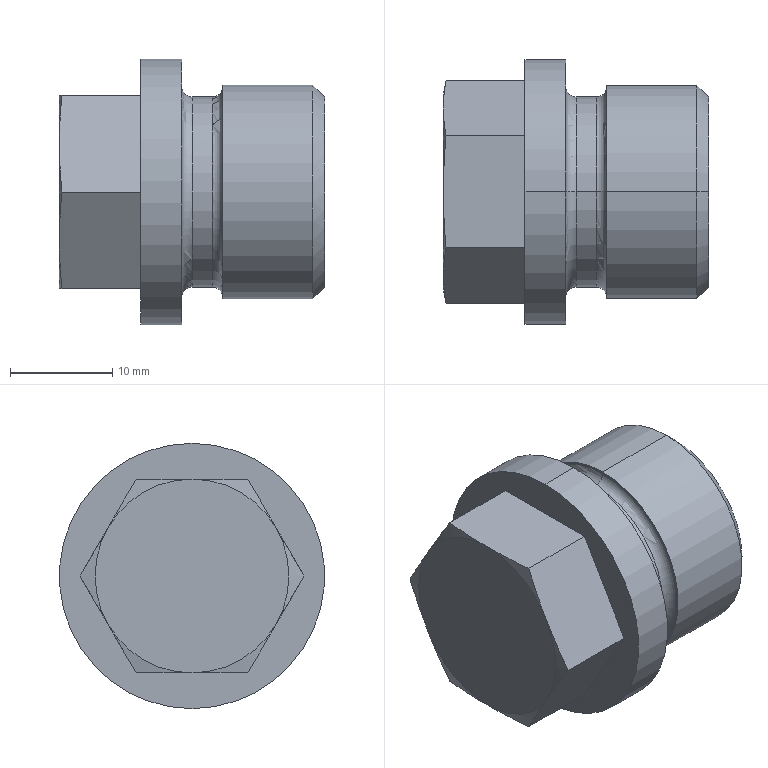Part | SolidWorks | features Boss 1, Cut 1, Fillet 1, Revolution 1 | 1 solid | 29 faces | box 26 x 26 x 26 mm | volume 9145 mm3 | plane 11 | cone 8 | cylinder 6 | torus 4 | commonest cylinder face diameters 18.631 x2 20.955 x2 26 x2
STEP:
#1=CARTESIAN_POINT('',(12.,0.,-10.316));
#2=VERTEX_POINT('',#1);
#3=CARTESIAN_POINT('',(12.,0.,10.316));
#4=VERTEX_POINT('',#3);
#5=CARTESIAN_POINT('',(12.,0.,0.));
#6=DIRECTION('',(-1.,0.,0.));
#7=DIRECTION('',(0.,0.,1.));
#8=AXIS2_PLACEMENT_3D('',#5,#6,#7);
#9=CIRCLE('',#8,10.316);
#10=EDGE_CURVE('',#2,#4,#9,.T.);
#11=ORIENTED_EDGE('',*,*,#10,.F.);
#12=CARTESIAN_POINT('',(13.,0.,-9.316));
#13=VERTEX_POINT('',#12);
#14=CARTESIAN_POINT('',(13.,0.,-10.316));
#15=DIRECTION('',(0.,1.,0.));
#16=DIRECTION('',(0.,0.,1.));
#17=AXIS2_PLACEMENT_3D('',#14,#15,#16);
#18=CIRCLE('',#17,1.);
#19=EDGE_CURVE('',#2,#13,#18,.T.);
#20=ORIENTED_EDGE('',*,*,#19,.T.);
#21=CARTESIAN_POINT('',(13.,0.,9.316));
#22=VERTEX_POINT('',#21);
#23=CARTESIAN_POINT('',(13.,0.,0.));
#24=DIRECTION('',(1.,0.,0.));
#25=DIRECTION('',(0.,0.,1.));
#26=AXIS2_PLACEMENT_3D('',#23,#24,#25);
#27=CIRCLE('',#26,9.316);
#28=EDGE_CURVE('',#22,#13,#27,.T.);
#29=ORIENTED_EDGE('',*,*,#28,.F.);
#30=CARTESIAN_POINT('',(13.,0.,10.316));
#31=DIRECTION('',(0.,-1.,0.));
#32=DIRECTION('',(0.,0.,-1.));
#33=AXIS2_PLACEMENT_3D('',#30,#31,#32);
#34=CIRCLE('',#33,1.);
#35=EDGE_CURVE('',#4,#22,#34,.T.);
#36=ORIENTED_EDGE('',*,*,#35,.F.);
#37=EDGE_LOOP('',(#11,#20,#29,#36));
#38=FACE_OUTER_BOUND('',#37,.T.);
#39=CARTESIAN_POINT('',(13.,0.,0.));
#40=DIRECTION('',(-1.,0.,0.));
#41=DIRECTION('',(0.,0.,1.));
#42=AXIS2_PLACEMENT_3D('',#39,#40,#41);
#43=TOROIDAL_SURFACE('',#42,10.316,1.);
#44=ADVANCED_FACE('',(#38),#43,.F.);
#45=CARTESIAN_POINT('',(16.,0.,10.316));
#46=VERTEX_POINT('',#45);
#47=CARTESIAN_POINT('',(16.,0.,-10.316));
#48=VERTEX_POINT('',#47);
#49=CARTESIAN_POINT('',(16.,0.,0.));
#50=DIRECTION('',(1.,0.,0.));
#51=DIRECTION('',(0.,0.,-1.));
#52=AXIS2_PLACEMENT_3D('',#49,#50,#51);
#53=CIRCLE('',#52,10.316);
#54=EDGE_CURVE('',#46,#48,#53,.T.);
#55=ORIENTED_EDGE('',*,*,#54,.F.);
#56=CARTESIAN_POINT('',(15.,0.,9.316));
#57=VERTEX_POINT('',#56);
#58=CARTESIAN_POINT('',(15.,0.,10.316));
#59=DIRECTION('',(0.,1.,0.));
#60=DIRECTION('',(0.,0.,1.));
#61=AXIS2_PLACEMENT_3D('',#58,#59,#60);
#62=CIRCLE('',#61,1.);
#63=EDGE_CURVE('',#46,#57,#62,.T.);
#64=ORIENTED_EDGE('',*,*,#63,.T.);
#65=CARTESIAN_POINT('',(15.,0.,-9.316));
#66=VERTEX_POINT('',#65);
#67=CARTESIAN_POINT('',(15.,0.,0.));
#68=DIRECTION('',(-1.,0.,0.));
#69=DIRECTION('',(0.,0.,-1.));
#70=AXIS2_PLACEMENT_3D('',#67,#68,#69);
#71=CIRCLE('',#70,9.316);
#72=EDGE_CURVE('',#66,#57,#71,.T.);
#73=ORIENTED_EDGE('',*,*,#72,.F.);
#74=CARTESIAN_POINT('',(15.,0.,-10.316));
#75=DIRECTION('',(0.,-1.,0.));
#76=DIRECTION('',(0.,0.,-1.));
#77=AXIS2_PLACEMENT_3D('',#74,#75,#76);
#78=CIRCLE('',#77,1.);
#79=EDGE_CURVE('',#48,#66,#78,.T.);
#80=ORIENTED_EDGE('',*,*,#79,.F.);
#81=EDGE_LOOP('',(#55,#64,#73,#80));
#82=FACE_OUTER_BOUND('',#81,.T.);
#83=CARTESIAN_POINT('',(15.,0.,0.));
#84=DIRECTION('',(1.,0.,0.));
#85=DIRECTION('',(0.,0.,-1.));
#86=AXIS2_PLACEMENT_3D('',#83,#84,#85);
#87=TOROIDAL_SURFACE('',#86,10.316,1.);
#88=ADVANCED_FACE('',(#82),#87,.F.);
#89=CARTESIAN_POINT('',(26.,0.,9.316));
#90=VERTEX_POINT('',#89);
#91=CARTESIAN_POINT('',(26.,0.,-9.316));
#92=VERTEX_POINT('',#91);
#93=CARTESIAN_POINT('',(26.,0.,0.));
#94=DIRECTION('',(-1.,0.,0.));
#95=DIRECTION('',(0.,0.,1.));
#96=AXIS2_PLACEMENT_3D('',#93,#94,#95);
#97=CIRCLE('',#96,9.316);
#98=EDGE_CURVE('',#90,#92,#97,.T.);
#99=ORIENTED_EDGE('',*,*,#98,.T.);
#100=CARTESIAN_POINT('',(24.838,0.,-10.477));
#101=VERTEX_POINT('',#100);
#102=CARTESIAN_POINT('',(26.,0.,-9.316));
#103=DIRECTION('',(-0.7071,0.,-0.7071));
#104=VECTOR('',#103,1000.);
#105=LINE('',#102,#104);
#106=EDGE_CURVE('',#92,#101,#105,.T.);
#107=ORIENTED_EDGE('',*,*,#106,.T.);
#108=CARTESIAN_POINT('',(24.838,0.,10.477));
#109=VERTEX_POINT('',#108);
#110=CARTESIAN_POINT('',(24.838,0.,0.));
#111=DIRECTION('',(-1.,0.,0.));
#112=DIRECTION('',(0.,0.,1.));
#113=AXIS2_PLACEMENT_3D('',#110,#111,#112);
#114=CIRCLE('',#113,10.477);
#115=EDGE_CURVE('',#109,#101,#114,.T.);
#116=ORIENTED_EDGE('',*,*,#115,.F.);
#117=CARTESIAN_POINT('',(26.,0.,9.316));
#118=DIRECTION('',(-0.7071,0.,0.7071));
#119=VECTOR('',#118,1000.);
#120=LINE('',#117,#119);
#121=EDGE_CURVE('',#90,#109,#120,.T.);
#122=ORIENTED_EDGE('',*,*,#121,.F.);
#123=EDGE_LOOP('',(#99,#107,#116,#122));
#124=FACE_OUTER_BOUND('',#123,.T.);
#125=CARTESIAN_POINT('',(26.,0.,0.));
#126=DIRECTION('',(-1.,0.,0.));
#127=DIRECTION('',(0.,0.,1.));
#128=AXIS2_PLACEMENT_3D('',#125,#126,#127);
#129=CONICAL_SURFACE('',#128,9.316,0.7854);
#130=ADVANCED_FACE('',(#124),#129,.T.);
#131=ORIENTED_EDGE('',*,*,#115,.T.);
#132=CARTESIAN_POINT('',(16.,0.,-10.477));
#133=VERTEX_POINT('',#132);
#134=CARTESIAN_POINT('',(0.,0.,-10.477));
#135=DIRECTION('',(-1.,0.,0.));
#136=VECTOR('',#135,1000.);
#137=LINE('',#134,#136);
#138=EDGE_CURVE('',#101,#133,#137,.T.);
#139=ORIENTED_EDGE('',*,*,#138,.T.);
#140=CARTESIAN_POINT('',(16.,0.,10.477));
#141=VERTEX_POINT('',#140);
#142=CARTESIAN_POINT('',(16.,0.,0.));
#143=DIRECTION('',(-1.,0.,0.));
#144=DIRECTION('',(0.,0.,1.));
#145=AXIS2_PLACEMENT_3D('',#142,#143,#144);
#146=CIRCLE('',#145,10.477);
#147=EDGE_CURVE('',#141,#133,#146,.T.);
#148=ORIENTED_EDGE('',*,*,#147,.F.);
#149=CARTESIAN_POINT('',(0.,0.,10.477));
#150=DIRECTION('',(-1.,0.,0.));
#151=VECTOR('',#150,1000.);
#152=LINE('',#149,#151);
#153=EDGE_CURVE('',#109,#141,#152,.T.);
#154=ORIENTED_EDGE('',*,*,#153,.F.);
#155=EDGE_LOOP('',(#131,#139,#148,#154));
#156=FACE_OUTER_BOUND('',#155,.T.);
#157=CARTESIAN_POINT('',(0.,0.,0.));
#158=DIRECTION('',(-1.,0.,0.));
#159=DIRECTION('',(0.,0.,1.));
#160=AXIS2_PLACEMENT_3D('',#157,#158,#159);
#161=CYLINDRICAL_SURFACE('',#160,10.477);
#162=ADVANCED_FACE('',(#156),#161,.T.);
#163=CARTESIAN_POINT('',(15.,0.,0.));
#164=DIRECTION('',(-1.,0.,0.));
#165=DIRECTION('',(0.,0.,-1.));
#166=AXIS2_PLACEMENT_3D('',#163,#164,#165);
#167=CIRCLE('',#166,9.316);
#168=EDGE_CURVE('',#57,#66,#167,.T.);
#169=ORIENTED_EDGE('',*,*,#168,.T.);
#170=CARTESIAN_POINT('',(0.,0.,-9.316));
#171=DIRECTION('',(-1.,0.,0.));
#172=VECTOR('',#171,1000.);
#173=LINE('',#170,#172);
#174=EDGE_CURVE('',#66,#13,#173,.T.);
#175=ORIENTED_EDGE('',*,*,#174,.T.);
#176=CARTESIAN_POINT('',(13.,0.,0.));
#177=DIRECTION('',(1.,0.,0.));
#178=DIRECTION('',(0.,0.,1.));
#179=AXIS2_PLACEMENT_3D('',#176,#177,#178);
#180=CIRCLE('',#179,9.316);
#181=EDGE_CURVE('',#13,#22,#180,.T.);
#182=ORIENTED_EDGE('',*,*,#181,.T.);
#183=CARTESIAN_POINT('',(0.,0.,9.316));
#184=DIRECTION('',(-1.,0.,0.));
#185=VECTOR('',#184,1000.);
#186=LINE('',#183,#185);
#187=EDGE_CURVE('',#57,#22,#186,.T.);
#188=ORIENTED_EDGE('',*,*,#187,.F.);
#189=EDGE_LOOP('',(#169,#175,#182,#188));
#190=FACE_OUTER_BOUND('',#189,.T.);
#191=CARTESIAN_POINT('',(0.,0.,0.));
#192=DIRECTION('',(-1.,0.,0.));
#193=DIRECTION('',(0.,0.,1.));
#194=AXIS2_PLACEMENT_3D('',#191,#192,#193);
#195=CYLINDRICAL_SURFACE('',#194,9.316);
#196=ADVANCED_FACE('',(#190),#195,.T.);
#197=CARTESIAN_POINT('',(12.,0.,13.));
#198=VERTEX_POINT('',#197);
#199=CARTESIAN_POINT('',(12.,0.,-13.));
#200=VERTEX_POINT('',#199);
#201=CARTESIAN_POINT('',(12.,0.,0.));
#202=DIRECTION('',(-1.,0.,0.));
#203=DIRECTION('',(0.,0.,1.));
#204=AXIS2_PLACEMENT_3D('',#201,#202,#203);
#205=CIRCLE('',#204,13.);
#206=EDGE_CURVE('',#198,#200,#205,.T.);
#207=ORIENTED_EDGE('',*,*,#206,.T.);
#208=CARTESIAN_POINT('',(8.,0.,-13.));
#209=VERTEX_POINT('',#208);
#210=CARTESIAN_POINT('',(0.,0.,-13.));
#211=DIRECTION('',(-1.,0.,0.));
#212=VECTOR('',#211,1000.);
#213=LINE('',#210,#212);
#214=EDGE_CURVE('',#200,#209,#213,.T.);
#215=ORIENTED_EDGE('',*,*,#214,.T.);
#216=CARTESIAN_POINT('',(8.,0.,13.));
#217=VERTEX_POINT('',#216);
#218=CARTESIAN_POINT('',(8.,0.,0.));
#219=DIRECTION('',(-1.,0.,0.));
#220=DIRECTION('',(0.,0.,1.));
#221=AXIS2_PLACEMENT_3D('',#218,#219,#220);
#222=CIRCLE('',#221,13.);
#223=EDGE_CURVE('',#217,#209,#222,.T.);
#224=ORIENTED_EDGE('',*,*,#223,.F.);
#225=CARTESIAN_POINT('',(0.,0.,13.));
#226=DIRECTION('',(-1.,0.,0.));
#227=VECTOR('',#226,1000.);
#228=LINE('',#225,#227);
#229=EDGE_CURVE('',#198,#217,#228,.T.);
#230=ORIENTED_EDGE('',*,*,#229,.F.);
#231=EDGE_LOOP('',(#207,#215,#224,#230));
#232=FACE_OUTER_BOUND('',#231,.T.);
#233=CARTESIAN_POINT('',(0.,0.,0.));
#234=DIRECTION('',(-1.,0.,0.));
#235=DIRECTION('',(0.,0.,1.));
#236=AXIS2_PLACEMENT_3D('',#233,#234,#235);
#237=CYLINDRICAL_SURFACE('',#236,13.);
#238=ADVANCED_FACE('',(#232),#237,.T.);
#239=CARTESIAN_POINT('',(8.,5.485,-9.5));
#240=VERTEX_POINT('',#239);
#241=CARTESIAN_POINT('',(0.2591,5.485,-9.5));
#242=VERTEX_POINT('',#241);
#243=CARTESIAN_POINT('',(37.023,5.485,-9.5));
#244=DIRECTION('',(-1.,0.,0.));
#245=VECTOR('',#244,1000.);
#246=LINE('',#243,#245);
#247=EDGE_CURVE('',#240,#242,#246,.T.);
#248=ORIENTED_EDGE('',*,*,#247,.T.);
#249=CARTESIAN_POINT('',(0.,8.227,-4.75));
#250=VERTEX_POINT('',#249);
#251=CARTESIAN_POINT('',(0.2591,5.485,-9.5));
#252=CARTESIAN_POINT('',(0.09795,6.399,-7.917));
#253=CARTESIAN_POINT('',(0.,7.313,-6.333));
#254=CARTESIAN_POINT('',(0.,8.227,-4.75));
#255=B_SPLINE_CURVE_WITH_KNOTS('',3,(#251,#252,#253,#254),.UNSPECIFIED.,.F.,.F.,(4,4),(0.000000231,0.005485),.UNSPECIFIED.);
#256=EDGE_CURVE('',#242,#250,#255,.T.);
#257=ORIENTED_EDGE('',*,*,#256,.T.);
#258=CARTESIAN_POINT('',(0.2591,10.97,0.));
#259=VERTEX_POINT('',#258);
#260=CARTESIAN_POINT('',(0.,8.227,-4.75));
#261=CARTESIAN_POINT('',(0.,9.141,-3.167));
#262=CARTESIAN_POINT('',(0.09795,10.056,-1.583));
#263=CARTESIAN_POINT('',(0.2591,10.97,0.));
#264=B_SPLINE_CURVE_WITH_KNOTS('',3,(#260,#261,#262,#263),.UNSPECIFIED.,.F.,.F.,(4,4),(0.005485,0.01097),.UNSPECIFIED.);
#265=EDGE_CURVE('',#250,#259,#264,.T.);
#266=ORIENTED_EDGE('',*,*,#265,.T.);
#267=CARTESIAN_POINT('',(8.,10.97,0.));
#268=VERTEX_POINT('',#267);
#269=CARTESIAN_POINT('',(37.023,10.97,0.));
#270=DIRECTION('',(-1.,0.,0.));
#271=VECTOR('',#270,1000.);
#272=LINE('',#269,#271);
#273=EDGE_CURVE('',#268,#259,#272,.T.);
#274=ORIENTED_EDGE('',*,*,#273,.F.);
#275=CARTESIAN_POINT('',(8.,10.97,0.));
#276=DIRECTION('',(0.,-0.5,-0.866));
#277=VECTOR('',#276,1000.);
#278=LINE('',#275,#277);
#279=EDGE_CURVE('',#268,#240,#278,.T.);
#280=ORIENTED_EDGE('',*,*,#279,.T.);
#281=EDGE_LOOP('',(#248,#257,#266,#274,#280));
#282=FACE_OUTER_BOUND('',#281,.T.);
#283=CARTESIAN_POINT('',(37.023,10.97,0.));
#284=DIRECTION('',(0.,0.866,-0.5));
#285=DIRECTION('',(0.,0.5,0.866));
#286=AXIS2_PLACEMENT_3D('',#283,#284,#285);
#287=PLANE('',#286);
#288=ADVANCED_FACE('',(#282),#287,.T.);
#289=CARTESIAN_POINT('',(8.,-5.485,-9.5));
#290=VERTEX_POINT('',#289);
#291=CARTESIAN_POINT('',(0.2591,-5.485,-9.5));
#292=VERTEX_POINT('',#291);
#293=CARTESIAN_POINT('',(37.023,-5.485,-9.5));
#294=DIRECTION('',(-1.,0.,0.));
#295=VECTOR('',#294,1000.);
#296=LINE('',#293,#295);
#297=EDGE_CURVE('',#290,#292,#296,.T.);
#298=ORIENTED_EDGE('',*,*,#297,.T.);
#299=CARTESIAN_POINT('',(0.,0.,-9.5));
#300=VERTEX_POINT('',#299);
#301=CARTESIAN_POINT('',(0.2591,-5.485,-9.5));
#302=CARTESIAN_POINT('',(0.1786,-4.572,-9.5));
#303=CARTESIAN_POINT('',(0.1131,-3.657,-9.5));
#304=CARTESIAN_POINT('',(0.02367,-1.828,-9.5));
#305=CARTESIAN_POINT('',(0.,-0.9137,-9.5));
#306=CARTESIAN_POINT('',(0.,0.,-9.5));
#307=B_SPLINE_CURVE_WITH_KNOTS('',3,(#301,#302,#303,#304,#305,#306),.UNSPECIFIED.,.F.,.F.,(4,2,4),(0.00925,0.012,0.01475),.UNSPECIFIED.);
#308=EDGE_CURVE('',#292,#300,#307,.T.);
#309=ORIENTED_EDGE('',*,*,#308,.T.);
#310=CARTESIAN_POINT('',(0.,0.,-9.5));
#311=CARTESIAN_POINT('',(0.,1.83,-9.5));
#312=CARTESIAN_POINT('',(0.09806,3.658,-9.5));
#313=CARTESIAN_POINT('',(0.2591,5.485,-9.5));
#314=B_SPLINE_CURVE_WITH_KNOTS('',3,(#310,#311,#312,#313),.UNSPECIFIED.,.F.,.F.,(4,4),(0.01475,0.02025),.UNSPECIFIED.);
#315=EDGE_CURVE('',#300,#242,#314,.T.);
#316=ORIENTED_EDGE('',*,*,#315,.T.);
#317=ORIENTED_EDGE('',*,*,#247,.F.);
#318=CARTESIAN_POINT('',(8.,5.485,-9.5));
#319=DIRECTION('',(0.,-1.,0.));
#320=VECTOR('',#319,1000.);
#321=LINE('',#318,#320);
#322=EDGE_CURVE('',#240,#290,#321,.T.);
#323=ORIENTED_EDGE('',*,*,#322,.T.);
#324=EDGE_LOOP('',(#298,#309,#316,#317,#323));
#325=FACE_OUTER_BOUND('',#324,.T.);
#326=CARTESIAN_POINT('',(37.023,5.485,-9.5));
#327=DIRECTION('',(0.,0.,-1.));
#328=DIRECTION('',(-1.,0.,0.));
#329=AXIS2_PLACEMENT_3D('',#326,#327,#328);
#330=PLANE('',#329);
#331=ADVANCED_FACE('',(#325),#330,.T.);
#332=CARTESIAN_POINT('',(8.,-10.97,0.));
#333=VERTEX_POINT('',#332);
#334=CARTESIAN_POINT('',(0.2591,-10.97,0.));
#335=VERTEX_POINT('',#334);
#336=CARTESIAN_POINT('',(37.023,-10.97,0.));
#337=DIRECTION('',(-1.,0.,0.));
#338=VECTOR('',#337,1000.);
#339=LINE('',#336,#338);
#340=EDGE_CURVE('',#333,#335,#339,.T.);
#341=ORIENTED_EDGE('',*,*,#340,.T.);
#342=CARTESIAN_POINT('',(0.,-8.227,-4.75));
#343=VERTEX_POINT('',#342);
#344=CARTESIAN_POINT('',(0.2591,-10.97,0.));
#345=CARTESIAN_POINT('',(0.09795,-10.056,-1.583));
#346=CARTESIAN_POINT('',(0.,-9.141,-3.167));
#347=CARTESIAN_POINT('',(0.,-8.227,-4.75));
#348=B_SPLINE_CURVE_WITH_KNOTS('',3,(#344,#345,#346,#347),.UNSPECIFIED.,.F.,.F.,(4,4),(0.000000231,0.005485),.UNSPECIFIED.);
#349=EDGE_CURVE('',#335,#343,#348,.T.);
#350=ORIENTED_EDGE('',*,*,#349,.T.);
#351=CARTESIAN_POINT('',(0.,-8.227,-4.75));
#352=CARTESIAN_POINT('',(0.,-7.313,-6.333));
#353=CARTESIAN_POINT('',(0.09795,-6.399,-7.917));
#354=CARTESIAN_POINT('',(0.2591,-5.485,-9.5));
#355=B_SPLINE_CURVE_WITH_KNOTS('',3,(#351,#352,#353,#354),.UNSPECIFIED.,.F.,.F.,(4,4),(0.005485,0.01097),.UNSPECIFIED.);
#356=EDGE_CURVE('',#343,#292,#355,.T.);
#357=ORIENTED_EDGE('',*,*,#356,.T.);
#358=ORIENTED_EDGE('',*,*,#297,.F.);
#359=CARTESIAN_POINT('',(8.,-5.485,-9.5));
#360=DIRECTION('',(0.,-0.5,0.866));
#361=VECTOR('',#360,1000.);
#362=LINE('',#359,#361);
#363=EDGE_CURVE('',#290,#333,#362,.T.);
#364=ORIENTED_EDGE('',*,*,#363,.T.);
#365=EDGE_LOOP('',(#341,#350,#357,#358,#364));
#366=FACE_OUTER_BOUND('',#365,.T.);
#367=CARTESIAN_POINT('',(37.023,-5.485,-9.5));
#368=DIRECTION('',(0.,-0.866,-0.5));
#369=DIRECTION('',(0.,0.5,-0.866));
#370=AXIS2_PLACEMENT_3D('',#367,#368,#369);
#371=PLANE('',#370);
#372=ADVANCED_FACE('',(#366),#371,.T.);
#373=CARTESIAN_POINT('',(8.,-5.485,9.5));
#374=VERTEX_POINT('',#373);
#375=CARTESIAN_POINT('',(0.2591,-5.485,9.5));
#376=VERTEX_POINT('',#375);
#377=CARTESIAN_POINT('',(37.023,-5.485,9.5));
#378=DIRECTION('',(-1.,0.,0.));
#379=VECTOR('',#378,1000.);
#380=LINE('',#377,#379);
#381=EDGE_CURVE('',#374,#376,#380,.T.);
#382=ORIENTED_EDGE('',*,*,#381,.T.);
#383=CARTESIAN_POINT('',(0.,-8.227,4.75));
#384=VERTEX_POINT('',#383);
#385=CARTESIAN_POINT('',(0.2591,-5.485,9.5));
#386=CARTESIAN_POINT('',(0.09795,-6.399,7.917));
#387=CARTESIAN_POINT('',(0.,-7.313,6.333));
#388=CARTESIAN_POINT('',(0.,-8.227,4.75));
#389=B_SPLINE_CURVE_WITH_KNOTS('',3,(#385,#386,#387,#388),.UNSPECIFIED.,.F.,.F.,(4,4),(0.000000231,0.005485),.UNSPECIFIED.);
#390=EDGE_CURVE('',#376,#384,#389,.T.);
#391=ORIENTED_EDGE('',*,*,#390,.T.);
#392=CARTESIAN_POINT('',(0.,-8.227,4.75));
#393=CARTESIAN_POINT('',(0.,-9.141,3.167));
#394=CARTESIAN_POINT('',(0.09795,-10.056,1.583));
#395=CARTESIAN_POINT('',(0.2591,-10.97,0.));
#396=B_SPLINE_CURVE_WITH_KNOTS('',3,(#392,#393,#394,#395),.UNSPECIFIED.,.F.,.F.,(4,4),(0.005485,0.01097),.UNSPECIFIED.);
#397=EDGE_CURVE('',#384,#335,#396,.T.);
#398=ORIENTED_EDGE('',*,*,#397,.T.);
#399=ORIENTED_EDGE('',*,*,#340,.F.);
#400=CARTESIAN_POINT('',(8.,-10.97,0.));
#401=DIRECTION('',(0.,0.5,0.866));
#402=VECTOR('',#401,1000.);
#403=LINE('',#400,#402);
#404=EDGE_CURVE('',#333,#374,#403,.T.);
#405=ORIENTED_EDGE('',*,*,#404,.T.);
#406=EDGE_LOOP('',(#382,#391,#398,#399,#405));
#407=FACE_OUTER_BOUND('',#406,.T.);
#408=CARTESIAN_POINT('',(37.023,-10.97,0.));
#409=DIRECTION('',(0.,-0.866,0.5));
#410=DIRECTION('',(0.,-0.5,-0.866));
#411=AXIS2_PLACEMENT_3D('',#408,#409,#410);
#412=PLANE('',#411);
#413=ADVANCED_FACE('',(#407),#412,.T.);
#414=CARTESIAN_POINT('',(8.,5.485,9.5));
#415=VERTEX_POINT('',#414);
#416=CARTESIAN_POINT('',(0.2591,5.485,9.5));
#417=VERTEX_POINT('',#416);
#418=CARTESIAN_POINT('',(37.023,5.485,9.5));
#419=DIRECTION('',(-1.,0.,0.));
#420=VECTOR('',#419,1000.);
#421=LINE('',#418,#420);
#422=EDGE_CURVE('',#415,#417,#421,.T.);
#423=ORIENTED_EDGE('',*,*,#422,.T.);
#424=CARTESIAN_POINT('',(0.,0.,9.5));
#425=VERTEX_POINT('',#424);
#426=CARTESIAN_POINT('',(0.2591,5.485,9.5));
#427=CARTESIAN_POINT('',(0.09806,3.658,9.5));
#428=CARTESIAN_POINT('',(0.,1.83,9.5));
#429=CARTESIAN_POINT('',(0.,0.,9.5));
#430=B_SPLINE_CURVE_WITH_KNOTS('',3,(#426,#427,#428,#429),.UNSPECIFIED.,.F.,.F.,(4,4),(0.02674,0.03224),.UNSPECIFIED.);
#431=EDGE_CURVE('',#417,#425,#430,.T.);
#432=ORIENTED_EDGE('',*,*,#431,.T.);
#433=CARTESIAN_POINT('',(0.,0.,9.5));
#434=CARTESIAN_POINT('',(0.,-0.9137,9.5));
#435=CARTESIAN_POINT('',(0.02367,-1.828,9.5));
#436=CARTESIAN_POINT('',(0.1131,-3.657,9.5));
#437=CARTESIAN_POINT('',(0.1786,-4.572,9.5));
#438=CARTESIAN_POINT('',(0.2591,-5.485,9.5));
#439=B_SPLINE_CURVE_WITH_KNOTS('',3,(#433,#434,#435,#436,#437,#438),.UNSPECIFIED.,.F.,.F.,(4,2,4),(0.03224,0.03499,0.03773),.UNSPECIFIED.);
#440=EDGE_CURVE('',#425,#376,#439,.T.);
#441=ORIENTED_EDGE('',*,*,#440,.T.);
#442=ORIENTED_EDGE('',*,*,#381,.F.);
#443=CARTESIAN_POINT('',(8.,-5.485,9.5));
#444=DIRECTION('',(0.,1.,0.));
#445=VECTOR('',#444,1000.);
#446=LINE('',#443,#445);
#447=EDGE_CURVE('',#374,#415,#446,.T.);
#448=ORIENTED_EDGE('',*,*,#447,.T.);
#449=EDGE_LOOP('',(#423,#432,#441,#442,#448));
#450=FACE_OUTER_BOUND('',#449,.T.);
#451=CARTESIAN_POINT('',(37.023,-5.485,9.5));
#452=DIRECTION('',(0.,0.,1.));
#453=DIRECTION('',(0.,-1.,0.));
#454=AXIS2_PLACEMENT_3D('',#451,#452,#453);
#455=PLANE('',#454);
#456=ADVANCED_FACE('',(#450),#455,.T.);
#457=ORIENTED_EDGE('',*,*,#273,.T.);
#458=CARTESIAN_POINT('',(0.,8.227,4.75));
#459=VERTEX_POINT('',#458);
#460=CARTESIAN_POINT('',(0.2591,10.97,0.));
#461=CARTESIAN_POINT('',(0.09795,10.056,1.583));
#462=CARTESIAN_POINT('',(0.,9.141,3.167));
#463=CARTESIAN_POINT('',(0.,8.227,4.75));
#464=B_SPLINE_CURVE_WITH_KNOTS('',3,(#460,#461,#462,#463),.UNSPECIFIED.,.F.,.F.,(4,4),(0.000000231,0.005485),.UNSPECIFIED.);
#465=EDGE_CURVE('',#259,#459,#464,.T.);
#466=ORIENTED_EDGE('',*,*,#465,.T.);
#467=CARTESIAN_POINT('',(0.,8.227,4.75));
#468=CARTESIAN_POINT('',(0.,7.313,6.333));
#469=CARTESIAN_POINT('',(0.09795,6.399,7.917));
#470=CARTESIAN_POINT('',(0.2591,5.485,9.5));
#471=B_SPLINE_CURVE_WITH_KNOTS('',3,(#467,#468,#469,#470),.UNSPECIFIED.,.F.,.F.,(4,4),(0.005485,0.01097),.UNSPECIFIED.);
#472=EDGE_CURVE('',#459,#417,#471,.T.);
#473=ORIENTED_EDGE('',*,*,#472,.T.);
#474=ORIENTED_EDGE('',*,*,#422,.F.);
#475=CARTESIAN_POINT('',(8.,5.485,9.5));
#476=DIRECTION('',(0.,0.5,-0.866));
#477=VECTOR('',#476,1000.);
#478=LINE('',#475,#477);
#479=EDGE_CURVE('',#415,#268,#478,.T.);
#480=ORIENTED_EDGE('',*,*,#479,.T.);
#481=EDGE_LOOP('',(#457,#466,#473,#474,#480));
#482=FACE_OUTER_BOUND('',#481,.T.);
#483=CARTESIAN_POINT('',(37.023,5.485,9.5));
#484=DIRECTION('',(0.,0.866,0.5));
#485=DIRECTION('',(0.,-0.5,0.866));
#486=AXIS2_PLACEMENT_3D('',#483,#484,#485);
#487=PLANE('',#486);
#488=ADVANCED_FACE('',(#482),#487,.T.);
#489=ORIENTED_EDGE('',*,*,#322,.F.);
#490=ORIENTED_EDGE('',*,*,#279,.F.);
#491=ORIENTED_EDGE('',*,*,#479,.F.);
#492=ORIENTED_EDGE('',*,*,#447,.F.);
#493=ORIENTED_EDGE('',*,*,#404,.F.);
#494=ORIENTED_EDGE('',*,*,#363,.F.);
#495=EDGE_LOOP('',(#489,#490,#491,#492,#493,#494));
#496=FACE_BOUND('',#495,.T.);
#497=ORIENTED_EDGE('',*,*,#223,.T.);
#498=CARTESIAN_POINT('',(8.,0.,0.));
#499=DIRECTION('',(-1.,0.,0.));
#500=DIRECTION('',(0.,0.,1.));
#501=AXIS2_PLACEMENT_3D('',#498,#499,#500);
#502=CIRCLE('',#501,13.);
#503=EDGE_CURVE('',#209,#217,#502,.T.);
#504=ORIENTED_EDGE('',*,*,#503,.T.);
#505=EDGE_LOOP('',(#497,#504));
#506=FACE_OUTER_BOUND('',#505,.T.);
#507=CARTESIAN_POINT('',(8.,13.,0.));
#508=DIRECTION('',(1.,0.,0.));
#509=DIRECTION('',(0.,0.,-1.));
#510=AXIS2_PLACEMENT_3D('',#507,#508,#509);
#511=PLANE('',#510);
#512=ADVANCED_FACE('',(#496,#506),#511,.F.);
#513=ORIENTED_EDGE('',*,*,#214,.F.);
#514=CARTESIAN_POINT('',(12.,0.,0.));
#515=DIRECTION('',(-1.,0.,0.));
#516=DIRECTION('',(0.,0.,1.));
#517=AXIS2_PLACEMENT_3D('',#514,#515,#516);
#518=CIRCLE('',#517,13.);
#519=EDGE_CURVE('',#200,#198,#518,.T.);
#520=ORIENTED_EDGE('',*,*,#519,.T.);
#521=ORIENTED_EDGE('',*,*,#229,.T.);
#522=ORIENTED_EDGE('',*,*,#503,.F.);
#523=EDGE_LOOP('',(#513,#520,#521,#522));
#524=FACE_OUTER_BOUND('',#523,.T.);
#525=CARTESIAN_POINT('',(0.,0.,0.));
#526=DIRECTION('',(-1.,0.,0.));
#527=DIRECTION('',(0.,0.,1.));
#528=AXIS2_PLACEMENT_3D('',#525,#526,#527);
#529=CYLINDRICAL_SURFACE('',#528,13.);
#530=ADVANCED_FACE('',(#524),#529,.T.);
#531=CARTESIAN_POINT('',(12.,0.,0.));
#532=DIRECTION('',(-1.,0.,0.));
#533=DIRECTION('',(0.,0.,1.));
#534=AXIS2_PLACEMENT_3D('',#531,#532,#533);
#535=CIRCLE('',#534,10.316);
#536=EDGE_CURVE('',#4,#2,#535,.T.);
#537=ORIENTED_EDGE('',*,*,#536,.T.);
#538=ORIENTED_EDGE('',*,*,#10,.T.);
#539=EDGE_LOOP('',(#537,#538));
#540=FACE_BOUND('',#539,.T.);
#541=ORIENTED_EDGE('',*,*,#206,.F.);
#542=ORIENTED_EDGE('',*,*,#519,.F.);
#543=EDGE_LOOP('',(#541,#542));
#544=FACE_OUTER_BOUND('',#543,.T.);
#545=CARTESIAN_POINT('',(12.,9.316,0.));
#546=DIRECTION('',(-1.,0.,0.));
#547=DIRECTION('',(0.,0.,1.));
#548=AXIS2_PLACEMENT_3D('',#545,#546,#547);
#549=PLANE('',#548);
#550=ADVANCED_FACE('',(#540,#544),#549,.F.);
#551=ORIENTED_EDGE('',*,*,#174,.F.);
#552=ORIENTED_EDGE('',*,*,#72,.T.);
#553=ORIENTED_EDGE('',*,*,#187,.T.);
#554=ORIENTED_EDGE('',*,*,#28,.T.);
#555=EDGE_LOOP('',(#551,#552,#553,#554));
#556=FACE_OUTER_BOUND('',#555,.T.);
#557=CARTESIAN_POINT('',(0.,0.,0.));
#558=DIRECTION('',(-1.,0.,0.));
#559=DIRECTION('',(0.,0.,1.));
#560=AXIS2_PLACEMENT_3D('',#557,#558,#559);
#561=CYLINDRICAL_SURFACE('',#560,9.316);
#562=ADVANCED_FACE('',(#556),#561,.T.);
#563=CARTESIAN_POINT('',(16.,0.,0.));
#564=DIRECTION('',(1.,0.,0.));
#565=DIRECTION('',(0.,0.,-1.));
#566=AXIS2_PLACEMENT_3D('',#563,#564,#565);
#567=CIRCLE('',#566,10.316);
#568=EDGE_CURVE('',#48,#46,#567,.T.);
#569=ORIENTED_EDGE('',*,*,#568,.T.);
#570=ORIENTED_EDGE('',*,*,#54,.T.);
#571=EDGE_LOOP('',(#569,#570));
#572=FACE_BOUND('',#571,.T.);
#573=ORIENTED_EDGE('',*,*,#147,.T.);
#574=CARTESIAN_POINT('',(16.,0.,0.));
#575=DIRECTION('',(-1.,0.,0.));
#576=DIRECTION('',(0.,0.,1.));
#577=AXIS2_PLACEMENT_3D('',#574,#575,#576);
#578=CIRCLE('',#577,10.477);
#579=EDGE_CURVE('',#133,#141,#578,.T.);
#580=ORIENTED_EDGE('',*,*,#579,.T.);
#581=EDGE_LOOP('',(#573,#580));
#582=FACE_OUTER_BOUND('',#581,.T.);
#583=CARTESIAN_POINT('',(16.,10.477,0.));
#584=DIRECTION('',(1.,0.,0.));
#585=DIRECTION('',(0.,0.,-1.));
#586=AXIS2_PLACEMENT_3D('',#583,#584,#585);
#587=PLANE('',#586);
#588=ADVANCED_FACE('',(#572,#582),#587,.F.);
#589=ORIENTED_EDGE('',*,*,#138,.F.);
#590=CARTESIAN_POINT('',(24.838,0.,0.));
#591=DIRECTION('',(-1.,0.,0.));
#592=DIRECTION('',(0.,0.,1.));
#593=AXIS2_PLACEMENT_3D('',#590,#591,#592);
#594=CIRCLE('',#593,10.477);
#595=EDGE_CURVE('',#101,#109,#594,.T.);
#596=ORIENTED_EDGE('',*,*,#595,.T.);
#597=ORIENTED_EDGE('',*,*,#153,.T.);
#598=ORIENTED_EDGE('',*,*,#579,.F.);
#599=EDGE_LOOP('',(#589,#596,#597,#598));
#600=FACE_OUTER_BOUND('',#599,.T.);
#601=CARTESIAN_POINT('',(0.,0.,0.));
#602=DIRECTION('',(-1.,0.,0.));
#603=DIRECTION('',(0.,0.,1.));
#604=AXIS2_PLACEMENT_3D('',#601,#602,#603);
#605=CYLINDRICAL_SURFACE('',#604,10.477);
#606=ADVANCED_FACE('',(#600),#605,.T.);
#607=ORIENTED_EDGE('',*,*,#106,.F.);
#608=CARTESIAN_POINT('',(26.,0.,0.));
#609=DIRECTION('',(-1.,0.,0.));
#610=DIRECTION('',(0.,0.,1.));
#611=AXIS2_PLACEMENT_3D('',#608,#609,#610);
#612=CIRCLE('',#611,9.316);
#613=EDGE_CURVE('',#92,#90,#612,.T.);
#614=ORIENTED_EDGE('',*,*,#613,.T.);
#615=ORIENTED_EDGE('',*,*,#121,.T.);
#616=ORIENTED_EDGE('',*,*,#595,.F.);
#617=EDGE_LOOP('',(#607,#614,#615,#616));
#618=FACE_OUTER_BOUND('',#617,.T.);
#619=CARTESIAN_POINT('',(26.,0.,0.));
#620=DIRECTION('',(-1.,0.,0.));
#621=DIRECTION('',(0.,0.,1.));
#622=AXIS2_PLACEMENT_3D('',#619,#620,#621);
#623=CONICAL_SURFACE('',#622,9.316,0.7854);
#624=ADVANCED_FACE('',(#618),#623,.T.);
#625=ORIENTED_EDGE('',*,*,#98,.F.);
#626=ORIENTED_EDGE('',*,*,#613,.F.);
#627=EDGE_LOOP('',(#625,#626));
#628=FACE_OUTER_BOUND('',#627,.T.);
#629=CARTESIAN_POINT('',(26.,9.316,0.));
#630=DIRECTION('',(-1.,0.,0.));
#631=DIRECTION('',(0.,0.,1.));
#632=AXIS2_PLACEMENT_3D('',#629,#630,#631);
#633=PLANE('',#632);
#634=ADVANCED_FACE('',(#628),#633,.F.);
#635=CARTESIAN_POINT('',(0.,0.,0.));
#636=DIRECTION('',(1.,0.,0.));
#637=DIRECTION('',(0.,0.,-1.));
#638=AXIS2_PLACEMENT_3D('',#635,#636,#637);
#639=CIRCLE('',#638,9.5);
#640=EDGE_CURVE('',#343,#300,#639,.T.);
#641=ORIENTED_EDGE('',*,*,#640,.T.);
#642=ORIENTED_EDGE('',*,*,#308,.F.);
#643=ORIENTED_EDGE('',*,*,#356,.F.);
#644=EDGE_LOOP('',(#641,#642,#643));
#645=FACE_OUTER_BOUND('',#644,.T.);
#646=CARTESIAN_POINT('',(0.,0.,0.));
#647=DIRECTION('',(1.,0.,0.));
#648=DIRECTION('',(0.,0.,1.));
#649=AXIS2_PLACEMENT_3D('',#646,#647,#648);
#650=CONICAL_SURFACE('',#649,9.5,1.396);
#651=ADVANCED_FACE('',(#645),#650,.T.);
#652=ORIENTED_EDGE('',*,*,#397,.F.);
#653=CARTESIAN_POINT('',(0.,0.,0.));
#654=DIRECTION('',(1.,0.,0.));
#655=DIRECTION('',(0.,0.,-1.));
#656=AXIS2_PLACEMENT_3D('',#653,#654,#655);
#657=CIRCLE('',#656,9.5);
#658=EDGE_CURVE('',#384,#343,#657,.T.);
#659=ORIENTED_EDGE('',*,*,#658,.T.);
#660=ORIENTED_EDGE('',*,*,#349,.F.);
#661=EDGE_LOOP('',(#652,#659,#660));
#662=FACE_OUTER_BOUND('',#661,.T.);
#663=CARTESIAN_POINT('',(0.,0.,0.));
#664=DIRECTION('',(1.,0.,0.));
#665=DIRECTION('',(0.,0.,1.));
#666=AXIS2_PLACEMENT_3D('',#663,#664,#665);
#667=CONICAL_SURFACE('',#666,9.5,1.396);
#668=ADVANCED_FACE('',(#662),#667,.T.);
#669=ORIENTED_EDGE('',*,*,#440,.F.);
#670=CARTESIAN_POINT('',(0.,0.,0.));
#671=DIRECTION('',(1.,0.,0.));
#672=DIRECTION('',(0.,0.,-1.));
#673=AXIS2_PLACEMENT_3D('',#670,#671,#672);
#674=CIRCLE('',#673,9.5);
#675=EDGE_CURVE('',#425,#384,#674,.T.);
#676=ORIENTED_EDGE('',*,*,#675,.T.);
#677=ORIENTED_EDGE('',*,*,#390,.F.);
#678=EDGE_LOOP('',(#669,#676,#677));
#679=FACE_OUTER_BOUND('',#678,.T.);
#680=CARTESIAN_POINT('',(0.,0.,0.));
#681=DIRECTION('',(1.,0.,0.));
#682=DIRECTION('',(0.,0.,1.));
#683=AXIS2_PLACEMENT_3D('',#680,#681,#682);
#684=CONICAL_SURFACE('',#683,9.5,1.396);
#685=ADVANCED_FACE('',(#679),#684,.T.);
#686=ORIENTED_EDGE('',*,*,#472,.F.);
#687=CARTESIAN_POINT('',(0.,0.,0.));
#688=DIRECTION('',(-1.,0.,0.));
#689=DIRECTION('',(0.,0.,1.));
#690=AXIS2_PLACEMENT_3D('',#687,#688,#689);
#691=CIRCLE('',#690,9.5);
#692=EDGE_CURVE('',#425,#459,#691,.T.);
#693=ORIENTED_EDGE('',*,*,#692,.F.);
#694=ORIENTED_EDGE('',*,*,#431,.F.);
#695=EDGE_LOOP('',(#686,#693,#694));
#696=FACE_OUTER_BOUND('',#695,.T.);
#697=CARTESIAN_POINT('',(0.,0.,0.));
#698=DIRECTION('',(1.,0.,0.));
#699=DIRECTION('',(0.,0.,1.));
#700=AXIS2_PLACEMENT_3D('',#697,#698,#699);
#701=CONICAL_SURFACE('',#700,9.5,1.396);
#702=ADVANCED_FACE('',(#696),#701,.T.);
#703=CARTESIAN_POINT('',(0.,0.,0.));
#704=DIRECTION('',(1.,0.,0.));
#705=DIRECTION('',(0.,0.,-1.));
#706=AXIS2_PLACEMENT_3D('',#703,#704,#705);
#707=CIRCLE('',#706,9.5);
#708=EDGE_CURVE('',#250,#459,#707,.T.);
#709=ORIENTED_EDGE('',*,*,#708,.T.);
#710=ORIENTED_EDGE('',*,*,#465,.F.);
#711=ORIENTED_EDGE('',*,*,#265,.F.);
#712=EDGE_LOOP('',(#709,#710,#711));
#713=FACE_OUTER_BOUND('',#712,.T.);
#714=CARTESIAN_POINT('',(0.,0.,0.));
#715=DIRECTION('',(1.,0.,0.));
#716=DIRECTION('',(0.,0.,1.));
#717=AXIS2_PLACEMENT_3D('',#714,#715,#716);
#718=CONICAL_SURFACE('',#717,9.5,1.396);
#719=ADVANCED_FACE('',(#713),#718,.T.);
#720=CARTESIAN_POINT('',(0.,0.,0.));
#721=DIRECTION('',(1.,0.,0.));
#722=DIRECTION('',(0.,0.,-1.));
#723=AXIS2_PLACEMENT_3D('',#720,#721,#722);
#724=CIRCLE('',#723,9.5);
#725=EDGE_CURVE('',#300,#250,#724,.T.);
#726=ORIENTED_EDGE('',*,*,#725,.T.);
#727=ORIENTED_EDGE('',*,*,#256,.F.);
#728=ORIENTED_EDGE('',*,*,#315,.F.);
#729=EDGE_LOOP('',(#726,#727,#728));
#730=FACE_OUTER_BOUND('',#729,.T.);
#731=CARTESIAN_POINT('',(0.,0.,0.));
#732=DIRECTION('',(1.,0.,0.));
#733=DIRECTION('',(0.,0.,1.));
#734=AXIS2_PLACEMENT_3D('',#731,#732,#733);
#735=CONICAL_SURFACE('',#734,9.5,1.396);
#736=ADVANCED_FACE('',(#730),#735,.T.);
#737=ORIENTED_EDGE('',*,*,#725,.F.);
#738=ORIENTED_EDGE('',*,*,#640,.F.);
#739=ORIENTED_EDGE('',*,*,#658,.F.);
#740=ORIENTED_EDGE('',*,*,#675,.F.);
#741=ORIENTED_EDGE('',*,*,#692,.T.);
#742=ORIENTED_EDGE('',*,*,#708,.F.);
#743=EDGE_LOOP('',(#737,#738,#739,#740,#741,#742));
#744=FACE_OUTER_BOUND('',#743,.T.);
#745=CARTESIAN_POINT('',(0.,1.5,0.));
#746=DIRECTION('',(1.,0.,0.));
#747=DIRECTION('',(0.,0.,-1.));
#748=AXIS2_PLACEMENT_3D('',#745,#746,#747);
#749=PLANE('',#748);
#750=ADVANCED_FACE('',(#744),#749,.F.);
#751=ORIENTED_EDGE('',*,*,#63,.F.);
#752=ORIENTED_EDGE('',*,*,#568,.F.);
#753=ORIENTED_EDGE('',*,*,#79,.T.);
#754=ORIENTED_EDGE('',*,*,#168,.F.);
#755=EDGE_LOOP('',(#751,#752,#753,#754));
#756=FACE_OUTER_BOUND('',#755,.T.);
#757=CARTESIAN_POINT('',(15.,0.,0.));
#758=DIRECTION('',(1.,0.,0.));
#759=DIRECTION('',(0.,0.,-1.));
#760=AXIS2_PLACEMENT_3D('',#757,#758,#759);
#761=TOROIDAL_SURFACE('',#760,10.316,1.);
#762=ADVANCED_FACE('',(#756),#761,.F.);
#763=ORIENTED_EDGE('',*,*,#19,.F.);
#764=ORIENTED_EDGE('',*,*,#536,.F.);
#765=ORIENTED_EDGE('',*,*,#35,.T.);
#766=ORIENTED_EDGE('',*,*,#181,.F.);
#767=EDGE_LOOP('',(#763,#764,#765,#766));
#768=FACE_OUTER_BOUND('',#767,.T.);
#769=CARTESIAN_POINT('',(13.,0.,0.));
#770=DIRECTION('',(-1.,0.,0.));
#771=DIRECTION('',(0.,0.,1.));
#772=AXIS2_PLACEMENT_3D('',#769,#770,#771);
#773=TOROIDAL_SURFACE('',#772,10.316,1.);
#774=ADVANCED_FACE('',(#768),#773,.F.);
#775=CLOSED_SHELL('',(#44,#88,#130,#162,#196,#238,#288,#331,#372,#413,#456,#488,#512,#530,#550,#562,#588,#606,#624,#634,#651,#668,#685,#702,#719,#736,#750,#762,#774));
#776=MANIFOLD_SOLID_BREP('',#775);
#777=CARTESIAN_POINT('',(0.,0.,0.));
#778=DIRECTION('',(0.,0.,1.));
#779=DIRECTION('',(1.,0.,0.));
#780=AXIS2_PLACEMENT_3D('',#777,#778,#779);
#781=(LENGTH_UNIT()NAMED_UNIT(*)SI_UNIT(.MILLI.,.METRE.));
#782=UNCERTAINTY_MEASURE_WITH_UNIT(LENGTH_MEASURE(0.00001),#781,'','');
#783=(NAMED_UNIT(*)PLANE_ANGLE_UNIT()SI_UNIT($,.RADIAN.));
#784=(NAMED_UNIT(*)SI_UNIT($,.STERADIAN.)SOLID_ANGLE_UNIT());
#785=(GEOMETRIC_REPRESENTATION_CONTEXT(3)GLOBAL_UNCERTAINTY_ASSIGNED_CONTEXT((#782))GLOBAL_UNIT_ASSIGNED_CONTEXT((#781,#783,#784))REPRESENTATION_CONTEXT('',''));
#786=ADVANCED_BREP_SHAPE_REPRESENTATION('',(#776,#780),#785);